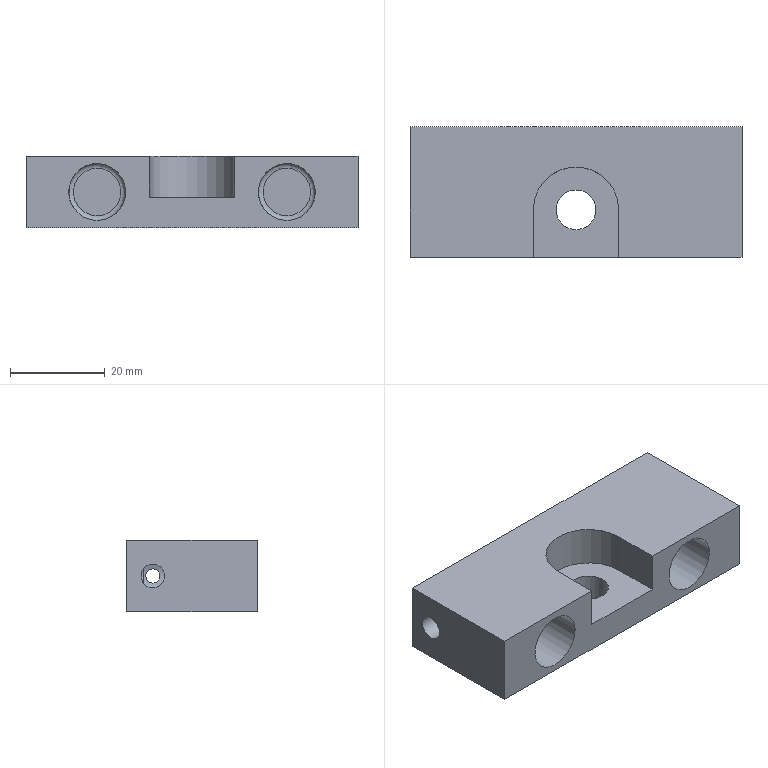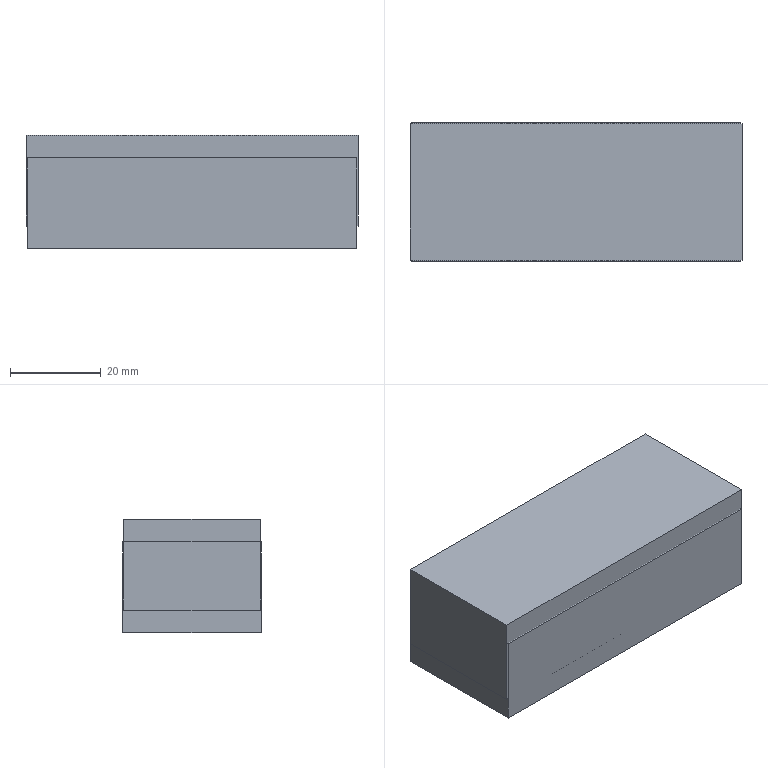CAM job | NX | 3+2 milling, drilling | part box 70 x 27.5 x 15 mm | stock box 73 x 30.5 x 25 mm
Tools:
number,name,description,diameter,corner_radius,flute_length,length,flutes
2,D10-30-D10-75-3T-ROUGH,D10-30-D10-75-3T-粗,10.0,0.0,30.0,75.0,2
4,D10-30-D10-75-3T-FINISH,D10-30-D10-75-3T,10.0,0.0,30.0,75.0,3
3,D4-12-D4-50-3T-ROUGH,D4-12-D4-50-3T-粗,4.0,0.0,12.0,50.0,2
5,倒角D4-90度,倒角D4-90度,4.0,0.0,5.0,50.0,2
1,D50面刀,D50面刀,30.0,0.0,30.0,30.0,4
7,点孔D10-90-90度,点孔D10-90-90度,10.0,0.0,0.0,90.0,2
9,钻头D3.0-42-71,钻刀D3.0-42-71,3.0,0.0,42.0,71.0,2
8,钻头D5.1-62-92,钻刀D5.1-62-92,5.1,0.0,62.0,92.0,2
10,上排M6-23-D6-63,上排M6-23-D6-63,6.0,0.0,23.0,26.0,2
0,点孔D10-150-90度,点孔D10-150-90度,10.0,0.0,0.0,150.0,2
0,钻头D11.5-106-143,钻刀D11.5-106-143,11.5,0.0,106.0,143.0,2
0,D8-25-D8-60-3T-ROUGH,D8-25-D8-60-3T-粗,8.0,0.0,25.0,60.0,2
0,D8R1,Milling Tool-5 Parameters,6.0,1.0,50.0,75.0,2
Operations:
program,operation,operation_type,tool,method,geometry_group,spindle_rpm,surface_speed,feed_per_tooth,feed_cut,feed_plunge,cut_length_mm,path_length_mm,cut_time_min,machine_time_min
A1,PLANAR_MILL_COPY,PlanarMilling,D50面刀,METHOD,A-G54,1600.0,150.0,0.125,800.0,100.0,136.0,169.9,0.17,0.1734
A1,ADAPTIVE_MILLING,CavityMilling,D10-30-D10-75-3T-ROUGH,METHOD,WORKPIECE_54,3000.0,94.0,0.25,1500.0,100.0,3597.809,3780.199,2.003,2.021
A1,PLANAR_MILL_4,PlanarMilling,D10-30-D10-75-3T-FINISH,METHOD,WORKPIECE_54,3000.0,94.0,0.0667,600.0,100.0,117.133,227.533,0.1952,0.2063
A1,PLANAR_MILL_1,PlanarMilling,D10-30-D10-75-3T-FINISH,METHOD,WORKPIECE_54,3000.0,94.0,0.0667,600.0,100.0,483.765,620.941,0.8063,0.82
A1,PLANAR_MILL_2,PlanarMilling,D4-12-D4-50-3T-ROUGH,METHOD,WORKPIECE_54,3000.0,37.0,0.1,600.0,100.0,495.818,558.418,0.8264,0.8326
A1,PLANAR_MILL_2_COPY,PlanarMilling,D4-12-D4-50-3T-ROUGH,METHOD,WORKPIECE_54,3000.0,37.0,0.05,300.0,100.0,35.938,103.538,0.1198,0.1266
A1,PLANAR_MILL_3,PlanarMilling,倒角D4-90度,METHOD,WORKPIECE_54,3000.0,37.0,0.1333,800.0,100.0,245.627,285.627,0.307,0.311
A1,PLANAR_MILL_3_COPY,PlanarMilling,倒角D4-90度,METHOD,WORKPIECE_54,3000.0,37.0,0.1333,800.0,100.0,22.038,79.238,0.0275,0.0333
A1,PLANAR_MILL_COPY_COPY,PlanarMilling,D50面刀,METHOD,A-G54,2500.0,235.0,0.06,600.0,100.0,136.0,170.0,0.2267,0.2301
B1,ADAPTIVE_MILLING_1,CavityMilling,D10-30-D10-75-3T-ROUGH,METHOD,WORKPIECE_55,3000.0,94.0,0.25,1500.0,100.0,7348.155,7381.955,4.899,4.902
B1,PLANAR_MILL_5,PlanarMilling,D50面刀,METHOD,WORKPIECE_55,1600.0,150.0,0.125,800.0,100.0,136.0,170.0,0.17,0.1734
B1,PLANAR_MILL_7,PlanarMilling,倒角D4-90度,METHOD,WORKPIECE_55,3000.0,37.0,0.1333,800.0,100.0,19.544,59.544,0.0244,0.0284
B1,PLANAR_MILL_6,PlanarMilling,倒角D4-90度,METHOD,WORKPIECE_55,3000.0,37.0,0.1333,800.0,100.0,217.353,255.353,0.2717,0.2755
C1,DRILLING,Operation,点孔D10-90-90度,METHOD,C-G56,1600.0,50.0,0.0469,150.0,0.0,4.5,49.0,0.03,0.0344
C1,DRILLING_1_COPY,Operation,钻头D5.1-62-92,METHOD,C-G56,1800.0,28.0,0.0417,150.0,0.0,18.0,76.0,0.12,0.1258
C1,DRILLING_1,Operation,钻头D3.0-42-71,METHOD,C-G56,1600.0,15.0,0.025,80.0,0.0,54.0,148.0,0.675,0.6844
C1,DRILLING_1_COPY_COPY,Operation,上排M6-23-D6-63,METHOD,C-G56,300.0,5.0,0.0017,1.0,0.0,8.0,56.0,8.0,8.005
D1,DRILLING_3,Operation,点孔D10-150-90度,METHOD,D-G57,1600.0,50.0,0.0469,150.0,0.0,4.5,49.0,0.03,0.0344
D1,DRILLING_2_COPY,Operation,钻头D5.1-62-92,METHOD,D-G57,1800.0,28.0,0.0417,150.0,0.0,23.0,86.0,0.1533,0.1596
D1,DRILLING_2_COPY_COPY,Operation,上排M6-23-D6-63,METHOD,D-G57,300.0,5.0,0.0017,1.0,0.0,8.0,56.0,8.0,8.005
E1,DRILLING_4,Operation,点孔D10-150-90度,METHOD,E-G58,1200.0,37.0,0.0417,100.0,0.0,9.0,101.112,0.09,0.0992
E1,DRILLING_5,Operation,钻头D11.5-106-143,METHOD,E-G58,600.0,21.0,0.0667,80.0,0.0,55.6,194.312,0.695,0.7089
E1,PLANAR_MILL_8,PlanarMilling,D8-25-D8-60-3T-ROUGH,METHOD,E-G58,2500.0,62.0,0.12,600.0,100.0,979.332,1141.73,1.632,1.649
E1,ZLEVEL_PROFILE_STEEP_1,ZLevelMilling,D8-25-D8-60-3T-ROUGH,METHOD,E-G58,2500.0,62.0,0.12,600.0,100.0,210.425,295.375,0.3507,0.3592
E1,ZLEVEL_PROFILE_STEEP_1_COPY,ZLevelMilling,D8-25-D8-60-3T-ROUGH,METHOD,E-G58,2500.0,62.0,0.12,600.0,100.0,210.424,295.374,0.3507,0.3592
E1,PLANAR_MILL_8_COPY,PlanarMilling,D8R1,METHOD,E-G58,2500.0,62.0,0.06,300.0,100.0,314.067,770.799,1.047,1.093
E1,PLANAR_MILL_9,PlanarMilling,D8R1,METHOD,E-G58,3000.0,56.0,0.05,300.0,100.0,83.417,296.798,0.2781,0.2994
E1,PLANAR_MILL_9_COPY,PlanarMilling,倒角D4-90度,METHOD,E-G58,3000.0,56.0,0.05,300.0,100.0,73.055,193.02,0.2435,0.2555